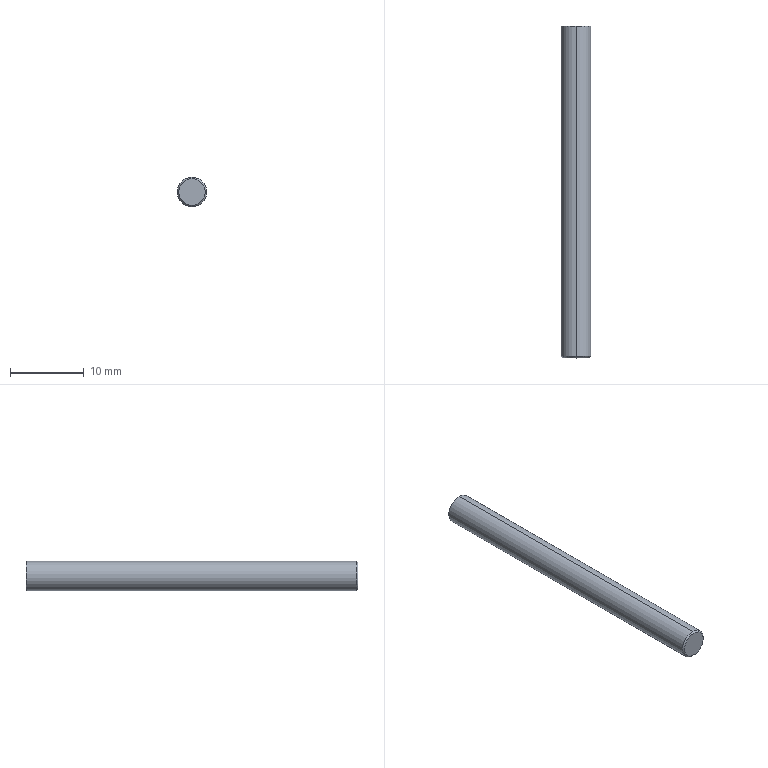Part | SolidWorks | features Chamfer 1, Extrusion 1, ICE 1 | 1 solid | 9 faces | box 4 x 45 x 4 mm | volume 544.038 mm3 | cylinder 4 | plane 3 | cone 2 | commonest cylinder face diameters 3 x2 4 x2
STEP:
#1=CARTESIAN_POINT('',(0.,42.,-1.5));
#2=VERTEX_POINT('',#1);
#3=CARTESIAN_POINT('',(0.,42.,1.5));
#4=VERTEX_POINT('',#3);
#5=CARTESIAN_POINT('',(0.,42.,0.));
#6=DIRECTION('',(0.,1.,0.));
#7=DIRECTION('',(0.,0.,1.));
#8=AXIS2_PLACEMENT_3D('',#5,#6,#7);
#9=CIRCLE('',#8,1.5);
#10=EDGE_CURVE('',#2,#4,#9,.T.);
#11=ORIENTED_EDGE('',*,*,#10,.F.);
#12=CARTESIAN_POINT('',(0.,45.,-1.5));
#13=VERTEX_POINT('',#12);
#14=CARTESIAN_POINT('',(0.,42.,-1.5));
#15=DIRECTION('',(0.,1.,0.));
#16=VECTOR('',#15,1000.);
#17=LINE('',#14,#16);
#18=EDGE_CURVE('',#2,#13,#17,.T.);
#19=ORIENTED_EDGE('',*,*,#18,.T.);
#20=CARTESIAN_POINT('',(0.,45.,1.5));
#21=VERTEX_POINT('',#20);
#22=CARTESIAN_POINT('',(0.,45.,0.));
#23=DIRECTION('',(0.,1.,0.));
#24=DIRECTION('',(0.,0.,1.));
#25=AXIS2_PLACEMENT_3D('',#22,#23,#24);
#26=CIRCLE('',#25,1.5);
#27=EDGE_CURVE('',#13,#21,#26,.T.);
#28=ORIENTED_EDGE('',*,*,#27,.T.);
#29=CARTESIAN_POINT('',(0.,42.,1.5));
#30=DIRECTION('',(0.,1.,0.));
#31=VECTOR('',#30,1000.);
#32=LINE('',#29,#31);
#33=EDGE_CURVE('',#4,#21,#32,.T.);
#34=ORIENTED_EDGE('',*,*,#33,.F.);
#35=EDGE_LOOP('',(#11,#19,#28,#34));
#36=FACE_OUTER_BOUND('',#35,.T.);
#37=CARTESIAN_POINT('',(0.,42.,0.));
#38=DIRECTION('',(0.,1.,0.));
#39=DIRECTION('',(0.,0.,1.));
#40=AXIS2_PLACEMENT_3D('',#37,#38,#39);
#41=CYLINDRICAL_SURFACE('',#40,1.5);
#42=ADVANCED_FACE('',(#36),#41,.F.);
#43=CARTESIAN_POINT('',(0.,0.,-1.8));
#44=VERTEX_POINT('',#43);
#45=CARTESIAN_POINT('',(0.,0.,1.8));
#46=VERTEX_POINT('',#45);
#47=CARTESIAN_POINT('',(0.,0.,0.));
#48=DIRECTION('',(0.,-1.,0.));
#49=DIRECTION('',(0.,0.,1.));
#50=AXIS2_PLACEMENT_3D('',#47,#48,#49);
#51=CIRCLE('',#50,1.8);
#52=EDGE_CURVE('',#44,#46,#51,.T.);
#53=ORIENTED_EDGE('',*,*,#52,.F.);
#54=CARTESIAN_POINT('',(0.,0.2,-2.));
#55=VERTEX_POINT('',#54);
#56=CARTESIAN_POINT('',(0.,0.2,-2.));
#57=DIRECTION('',(0.,0.7071,-0.7071));
#58=VECTOR('',#57,1000.);
#59=LINE('',#56,#58);
#60=EDGE_CURVE('',#44,#55,#59,.T.);
#61=ORIENTED_EDGE('',*,*,#60,.T.);
#62=CARTESIAN_POINT('',(0.,0.2,2.));
#63=VERTEX_POINT('',#62);
#64=CARTESIAN_POINT('',(0.,0.2,0.));
#65=DIRECTION('',(0.,1.,0.));
#66=DIRECTION('',(0.,0.,1.));
#67=AXIS2_PLACEMENT_3D('',#64,#65,#66);
#68=CIRCLE('',#67,2.);
#69=EDGE_CURVE('',#63,#55,#68,.T.);
#70=ORIENTED_EDGE('',*,*,#69,.F.);
#71=CARTESIAN_POINT('',(0.,0.2,2.));
#72=DIRECTION('',(0.,0.7071,0.7071));
#73=VECTOR('',#72,1000.);
#74=LINE('',#71,#73);
#75=EDGE_CURVE('',#46,#63,#74,.T.);
#76=ORIENTED_EDGE('',*,*,#75,.F.);
#77=EDGE_LOOP('',(#53,#61,#70,#76));
#78=FACE_OUTER_BOUND('',#77,.T.);
#79=CARTESIAN_POINT('',(0.,0.2,0.));
#80=DIRECTION('',(0.,1.,0.));
#81=DIRECTION('',(0.,0.,1.));
#82=AXIS2_PLACEMENT_3D('',#79,#80,#81);
#83=CONICAL_SURFACE('',#82,2.,0.7854);
#84=ADVANCED_FACE('',(#78),#83,.T.);
#85=CARTESIAN_POINT('',(0.,45.,2.));
#86=VERTEX_POINT('',#85);
#87=CARTESIAN_POINT('',(0.,45.,-2.));
#88=VERTEX_POINT('',#87);
#89=CARTESIAN_POINT('',(0.,45.,0.));
#90=DIRECTION('',(0.,1.,0.));
#91=DIRECTION('',(0.,0.,1.));
#92=AXIS2_PLACEMENT_3D('',#89,#90,#91);
#93=CIRCLE('',#92,2.);
#94=EDGE_CURVE('',#86,#88,#93,.T.);
#95=ORIENTED_EDGE('',*,*,#94,.F.);
#96=CARTESIAN_POINT('',(0.,45.,2.));
#97=DIRECTION('',(0.,-1.,0.));
#98=VECTOR('',#97,1000.);
#99=LINE('',#96,#98);
#100=EDGE_CURVE('',#86,#63,#99,.T.);
#101=ORIENTED_EDGE('',*,*,#100,.T.);
#102=ORIENTED_EDGE('',*,*,#69,.T.);
#103=CARTESIAN_POINT('',(0.,45.,-2.));
#104=DIRECTION('',(0.,-1.,0.));
#105=VECTOR('',#104,1000.);
#106=LINE('',#103,#105);
#107=EDGE_CURVE('',#88,#55,#106,.T.);
#108=ORIENTED_EDGE('',*,*,#107,.F.);
#109=EDGE_LOOP('',(#95,#101,#102,#108));
#110=FACE_OUTER_BOUND('',#109,.T.);
#111=CARTESIAN_POINT('',(0.,45.,0.));
#112=DIRECTION('',(0.,-1.,0.));
#113=DIRECTION('',(0.,0.,-1.));
#114=AXIS2_PLACEMENT_3D('',#111,#112,#113);
#115=CYLINDRICAL_SURFACE('',#114,2.);
#116=ADVANCED_FACE('',(#110),#115,.T.);
#117=ORIENTED_EDGE('',*,*,#100,.F.);
#118=CARTESIAN_POINT('',(0.,45.,0.));
#119=DIRECTION('',(0.,1.,0.));
#120=DIRECTION('',(0.,0.,1.));
#121=AXIS2_PLACEMENT_3D('',#118,#119,#120);
#122=CIRCLE('',#121,2.);
#123=EDGE_CURVE('',#88,#86,#122,.T.);
#124=ORIENTED_EDGE('',*,*,#123,.F.);
#125=ORIENTED_EDGE('',*,*,#107,.T.);
#126=CARTESIAN_POINT('',(0.,0.2,0.));
#127=DIRECTION('',(0.,1.,0.));
#128=DIRECTION('',(0.,0.,1.));
#129=AXIS2_PLACEMENT_3D('',#126,#127,#128);
#130=CIRCLE('',#129,2.);
#131=EDGE_CURVE('',#55,#63,#130,.T.);
#132=ORIENTED_EDGE('',*,*,#131,.T.);
#133=EDGE_LOOP('',(#117,#124,#125,#132));
#134=FACE_OUTER_BOUND('',#133,.T.);
#135=CARTESIAN_POINT('',(0.,45.,0.));
#136=DIRECTION('',(0.,-1.,0.));
#137=DIRECTION('',(0.,0.,-1.));
#138=AXIS2_PLACEMENT_3D('',#135,#136,#137);
#139=CYLINDRICAL_SURFACE('',#138,2.);
#140=ADVANCED_FACE('',(#134),#139,.T.);
#141=CARTESIAN_POINT('',(0.,45.,0.));
#142=DIRECTION('',(0.,1.,0.));
#143=DIRECTION('',(0.,0.,1.));
#144=AXIS2_PLACEMENT_3D('',#141,#142,#143);
#145=CIRCLE('',#144,1.5);
#146=EDGE_CURVE('',#21,#13,#145,.T.);
#147=ORIENTED_EDGE('',*,*,#146,.F.);
#148=ORIENTED_EDGE('',*,*,#27,.F.);
#149=EDGE_LOOP('',(#147,#148));
#150=FACE_BOUND('',#149,.T.);
#151=ORIENTED_EDGE('',*,*,#123,.T.);
#152=ORIENTED_EDGE('',*,*,#94,.T.);
#153=EDGE_LOOP('',(#151,#152));
#154=FACE_OUTER_BOUND('',#153,.T.);
#155=CARTESIAN_POINT('',(0.,45.,0.));
#156=DIRECTION('',(0.,1.,0.));
#157=DIRECTION('',(0.,0.,1.));
#158=AXIS2_PLACEMENT_3D('',#155,#156,#157);
#159=PLANE('',#158);
#160=ADVANCED_FACE('',(#150,#154),#159,.T.);
#161=CARTESIAN_POINT('',(0.,0.,0.));
#162=DIRECTION('',(0.,-1.,0.));
#163=DIRECTION('',(0.,0.,1.));
#164=AXIS2_PLACEMENT_3D('',#161,#162,#163);
#165=CIRCLE('',#164,1.8);
#166=EDGE_CURVE('',#46,#44,#165,.T.);
#167=ORIENTED_EDGE('',*,*,#166,.T.);
#168=ORIENTED_EDGE('',*,*,#52,.T.);
#169=EDGE_LOOP('',(#167,#168));
#170=FACE_OUTER_BOUND('',#169,.T.);
#171=CARTESIAN_POINT('',(0.,0.,0.));
#172=DIRECTION('',(0.,1.,0.));
#173=DIRECTION('',(0.,0.,1.));
#174=AXIS2_PLACEMENT_3D('',#171,#172,#173);
#175=PLANE('',#174);
#176=ADVANCED_FACE('',(#170),#175,.F.);
#177=ORIENTED_EDGE('',*,*,#60,.F.);
#178=ORIENTED_EDGE('',*,*,#166,.F.);
#179=ORIENTED_EDGE('',*,*,#75,.T.);
#180=ORIENTED_EDGE('',*,*,#131,.F.);
#181=EDGE_LOOP('',(#177,#178,#179,#180));
#182=FACE_OUTER_BOUND('',#181,.T.);
#183=CARTESIAN_POINT('',(0.,0.2,0.));
#184=DIRECTION('',(0.,1.,0.));
#185=DIRECTION('',(0.,0.,1.));
#186=AXIS2_PLACEMENT_3D('',#183,#184,#185);
#187=CONICAL_SURFACE('',#186,2.,0.7854);
#188=ADVANCED_FACE('',(#182),#187,.T.);
#189=ORIENTED_EDGE('',*,*,#18,.F.);
#190=CARTESIAN_POINT('',(0.,42.,0.));
#191=DIRECTION('',(0.,1.,0.));
#192=DIRECTION('',(0.,0.,1.));
#193=AXIS2_PLACEMENT_3D('',#190,#191,#192);
#194=CIRCLE('',#193,1.5);
#195=EDGE_CURVE('',#4,#2,#194,.T.);
#196=ORIENTED_EDGE('',*,*,#195,.F.);
#197=ORIENTED_EDGE('',*,*,#33,.T.);
#198=ORIENTED_EDGE('',*,*,#146,.T.);
#199=EDGE_LOOP('',(#189,#196,#197,#198));
#200=FACE_OUTER_BOUND('',#199,.T.);
#201=CARTESIAN_POINT('',(0.,42.,0.));
#202=DIRECTION('',(0.,1.,0.));
#203=DIRECTION('',(0.,0.,1.));
#204=AXIS2_PLACEMENT_3D('',#201,#202,#203);
#205=CYLINDRICAL_SURFACE('',#204,1.5);
#206=ADVANCED_FACE('',(#200),#205,.F.);
#207=ORIENTED_EDGE('',*,*,#195,.T.);
#208=ORIENTED_EDGE('',*,*,#10,.T.);
#209=EDGE_LOOP('',(#207,#208));
#210=FACE_OUTER_BOUND('',#209,.T.);
#211=CARTESIAN_POINT('',(0.,42.,0.));
#212=DIRECTION('',(0.,1.,0.));
#213=DIRECTION('',(0.,0.,1.));
#214=AXIS2_PLACEMENT_3D('',#211,#212,#213);
#215=PLANE('',#214);
#216=ADVANCED_FACE('',(#210),#215,.T.);
#217=CLOSED_SHELL('',(#42,#84,#116,#140,#160,#176,#188,#206,#216));
#218=MANIFOLD_SOLID_BREP('',#217);
#219=CARTESIAN_POINT('',(0.,0.,0.));
#220=DIRECTION('',(0.,0.,1.));
#221=DIRECTION('',(1.,0.,0.));
#222=AXIS2_PLACEMENT_3D('',#219,#220,#221);
#223=(LENGTH_UNIT()NAMED_UNIT(*)SI_UNIT(.MILLI.,.METRE.));
#224=UNCERTAINTY_MEASURE_WITH_UNIT(LENGTH_MEASURE(0.00001),#223,'','');
#225=(NAMED_UNIT(*)PLANE_ANGLE_UNIT()SI_UNIT($,.RADIAN.));
#226=(NAMED_UNIT(*)SI_UNIT($,.STERADIAN.)SOLID_ANGLE_UNIT());
#227=(GEOMETRIC_REPRESENTATION_CONTEXT(3)GLOBAL_UNCERTAINTY_ASSIGNED_CONTEXT((#224))GLOBAL_UNIT_ASSIGNED_CONTEXT((#223,#225,#226))REPRESENTATION_CONTEXT('',''));
#228=ADVANCED_BREP_SHAPE_REPRESENTATION('',(#218,#222),#227);